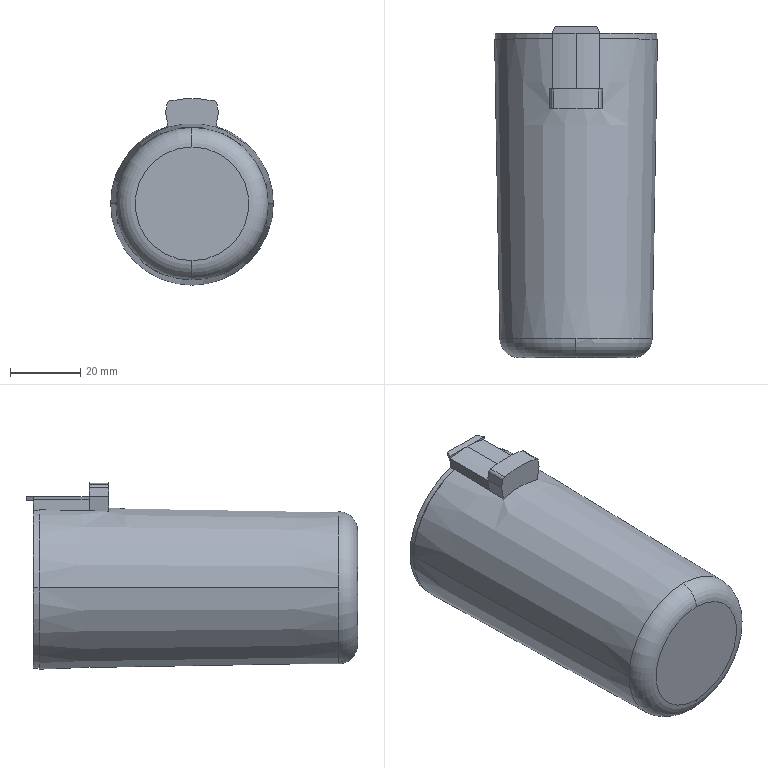Part | SolidWorks | features BaseBody 1 | 1 solid | 30 faces | box 46.4 x 94.4 x 53.2 mm | volume 146390 mm3 | plane 18 | cylinder 8 | torus 2 | cone 2 | commonest cylinder face diameters 46 x3 2 x2 51.98 x2 60 x1
STEP:
#1=CARTESIAN_POINT('',(21.709,-118.996,0.));
#2=VERTEX_POINT('',#1);
#3=CARTESIAN_POINT('',(0.,-118.996,21.709));
#4=VERTEX_POINT('',#3);
#5=CARTESIAN_POINT('',(0.,-118.996,0.));
#6=DIRECTION('',(0.,-1.,0.));
#7=DIRECTION('',(0.,0.,-1.));
#8=AXIS2_PLACEMENT_3D('',#5,#6,#7);
#9=CIRCLE('',#8,21.709);
#10=EDGE_CURVE('',#2,#4,#9,.T.);
#11=ORIENTED_EDGE('',*,*,#10,.T.);
#12=CARTESIAN_POINT('',(0.,-124.4,16.21));
#13=VERTEX_POINT('',#12);
#14=CARTESIAN_POINT('',(0.,-118.9,16.21));
#15=DIRECTION('',(1.,0.,0.));
#16=DIRECTION('',(0.,0.,-1.));
#17=AXIS2_PLACEMENT_3D('',#14,#15,#16);
#18=CIRCLE('',#17,5.5);
#19=EDGE_CURVE('',#4,#13,#18,.T.);
#20=ORIENTED_EDGE('',*,*,#19,.T.);
#21=CARTESIAN_POINT('',(0.,-124.4,-16.21));
#22=VERTEX_POINT('',#21);
#23=CARTESIAN_POINT('',(0.,-124.4,0.));
#24=DIRECTION('',(0.,-1.,0.));
#25=DIRECTION('',(0.,0.,-1.));
#26=AXIS2_PLACEMENT_3D('',#23,#24,#25);
#27=CIRCLE('',#26,16.21);
#28=EDGE_CURVE('',#22,#13,#27,.T.);
#29=ORIENTED_EDGE('',*,*,#28,.F.);
#30=CARTESIAN_POINT('',(0.,-118.996,-21.709));
#31=VERTEX_POINT('',#30);
#32=CARTESIAN_POINT('',(0.,-118.9,-16.21));
#33=DIRECTION('',(-1.,0.,0.));
#34=DIRECTION('',(0.,0.,1.));
#35=AXIS2_PLACEMENT_3D('',#32,#33,#34);
#36=CIRCLE('',#35,5.5);
#37=EDGE_CURVE('',#31,#22,#36,.T.);
#38=ORIENTED_EDGE('',*,*,#37,.F.);
#39=CARTESIAN_POINT('',(0.,-118.996,0.));
#40=DIRECTION('',(0.,-1.,0.));
#41=DIRECTION('',(0.,0.,-1.));
#42=AXIS2_PLACEMENT_3D('',#39,#40,#41);
#43=CIRCLE('',#42,21.709);
#44=EDGE_CURVE('',#31,#2,#43,.T.);
#45=ORIENTED_EDGE('',*,*,#44,.T.);
#46=EDGE_LOOP('',(#11,#20,#29,#38,#45));
#47=FACE_OUTER_BOUND('',#46,.T.);
#48=CARTESIAN_POINT('',(0.,-118.9,0.));
#49=DIRECTION('',(0.,-1.,0.));
#50=DIRECTION('',(0.,0.,-1.));
#51=AXIS2_PLACEMENT_3D('',#48,#49,#50);
#52=TOROIDAL_SURFACE('',#51,16.21,5.5);
#53=ADVANCED_FACE('',(#47),#52,.T.);
#54=ORIENTED_EDGE('',*,*,#10,.F.);
#55=CARTESIAN_POINT('',(23.2,-33.6,0.));
#56=VERTEX_POINT('',#55);
#57=CARTESIAN_POINT('',(23.2,-33.6,0.));
#58=DIRECTION('',(0.01745,0.9998,0.));
#59=VECTOR('',#58,1000.);
#60=LINE('',#57,#59);
#61=EDGE_CURVE('',#2,#56,#60,.T.);
#62=ORIENTED_EDGE('',*,*,#61,.T.);
#63=CARTESIAN_POINT('',(6.7,-33.6,22.211));
#64=VERTEX_POINT('',#63);
#65=CARTESIAN_POINT('',(0.,-33.6,0.));
#66=DIRECTION('',(0.,-1.,0.));
#67=DIRECTION('',(-0.2888,0.,0.9574));
#68=AXIS2_PLACEMENT_3D('',#65,#66,#67);
#69=CIRCLE('',#68,23.2);
#70=EDGE_CURVE('',#56,#64,#69,.T.);
#71=ORIENTED_EDGE('',*,*,#70,.T.);
#72=CARTESIAN_POINT('',(6.7,-47.862,21.951));
#73=VERTEX_POINT('',#72);
#74=CARTESIAN_POINT('',(6.7,-33.6,22.211));
#75=CARTESIAN_POINT('',(6.7,-38.354,22.125));
#76=CARTESIAN_POINT('',(6.7,-43.108,22.038));
#77=CARTESIAN_POINT('',(6.7,-47.862,21.951));
#78=B_SPLINE_CURVE_WITH_KNOTS('',3,(#74,#75,#76,#77),.UNSPECIFIED.,.F.,.F.,(4,4),(20.375,34.639),.UNSPECIFIED.);
#79=EDGE_CURVE('',#64,#73,#78,.T.);
#80=ORIENTED_EDGE('',*,*,#79,.T.);
#81=CARTESIAN_POINT('',(6.8,-47.862,21.92));
#82=VERTEX_POINT('',#81);
#83=CARTESIAN_POINT('',(0.,-47.862,0.));
#84=DIRECTION('',(0.,1.,0.));
#85=DIRECTION('',(0.2919,0.,0.9564));
#86=AXIS2_PLACEMENT_3D('',#83,#84,#85);
#87=CIRCLE('',#86,22.951);
#88=EDGE_CURVE('',#73,#82,#87,.T.);
#89=ORIENTED_EDGE('',*,*,#88,.T.);
#90=CARTESIAN_POINT('',(6.782,-53.5,21.823));
#91=VERTEX_POINT('',#90);
#92=CARTESIAN_POINT('',(6.782,-53.5,21.823));
#93=CARTESIAN_POINT('',(6.788,-51.621,21.855));
#94=CARTESIAN_POINT('',(6.794,-49.741,21.888));
#95=CARTESIAN_POINT('',(6.8,-47.862,21.92));
#96=B_SPLINE_CURVE_WITH_KNOTS('',3,(#92,#93,#94,#95),.UNSPECIFIED.,.F.,.F.,(4,4),(0.0002,5.639),.UNSPECIFIED.);
#97=EDGE_CURVE('',#91,#82,#96,.T.);
#98=ORIENTED_EDGE('',*,*,#97,.F.);
#99=CARTESIAN_POINT('',(-6.782,-53.5,21.823));
#100=VERTEX_POINT('',#99);
#101=CARTESIAN_POINT('',(0.,-53.5,0.));
#102=DIRECTION('',(0.,1.,0.));
#103=DIRECTION('',(-0.2968,0.,0.9549));
#104=AXIS2_PLACEMENT_3D('',#101,#102,#103);
#105=CIRCLE('',#104,22.853);
#106=EDGE_CURVE('',#100,#91,#105,.T.);
#107=ORIENTED_EDGE('',*,*,#106,.F.);
#108=CARTESIAN_POINT('',(-6.8,-47.862,21.92));
#109=VERTEX_POINT('',#108);
#110=CARTESIAN_POINT('',(-6.8,-47.862,21.92));
#111=CARTESIAN_POINT('',(-6.794,-49.741,21.888));
#112=CARTESIAN_POINT('',(-6.788,-51.621,21.855));
#113=CARTESIAN_POINT('',(-6.782,-53.5,21.823));
#114=B_SPLINE_CURVE_WITH_KNOTS('',3,(#110,#111,#112,#113),.UNSPECIFIED.,.F.,.F.,(4,4),(0.0002,5.639),.UNSPECIFIED.);
#115=EDGE_CURVE('',#109,#100,#114,.T.);
#116=ORIENTED_EDGE('',*,*,#115,.F.);
#117=CARTESIAN_POINT('',(-6.7,-47.862,21.951));
#118=VERTEX_POINT('',#117);
#119=CARTESIAN_POINT('',(0.,-47.862,0.));
#120=DIRECTION('',(0.,1.,0.));
#121=DIRECTION('',(-0.2963,0.,0.9551));
#122=AXIS2_PLACEMENT_3D('',#119,#120,#121);
#123=CIRCLE('',#122,22.951);
#124=EDGE_CURVE('',#109,#118,#123,.T.);
#125=ORIENTED_EDGE('',*,*,#124,.T.);
#126=CARTESIAN_POINT('',(-6.7,-33.6,22.211));
#127=VERTEX_POINT('',#126);
#128=CARTESIAN_POINT('',(-6.7,-47.862,21.951));
#129=CARTESIAN_POINT('',(-6.7,-43.108,22.038));
#130=CARTESIAN_POINT('',(-6.7,-38.354,22.125));
#131=CARTESIAN_POINT('',(-6.7,-33.6,22.211));
#132=B_SPLINE_CURVE_WITH_KNOTS('',3,(#128,#129,#130,#131),.UNSPECIFIED.,.F.,.F.,(4,4),(26.014,40.278),.UNSPECIFIED.);
#133=EDGE_CURVE('',#118,#127,#132,.T.);
#134=ORIENTED_EDGE('',*,*,#133,.T.);
#135=CARTESIAN_POINT('',(-23.2,-33.6,0.));
#136=VERTEX_POINT('',#135);
#137=CARTESIAN_POINT('',(0.,-33.6,0.));
#138=DIRECTION('',(0.,-1.,0.));
#139=DIRECTION('',(-0.2888,0.,0.9574));
#140=AXIS2_PLACEMENT_3D('',#137,#138,#139);
#141=CIRCLE('',#140,23.2);
#142=EDGE_CURVE('',#127,#136,#141,.T.);
#143=ORIENTED_EDGE('',*,*,#142,.T.);
#144=CARTESIAN_POINT('',(-21.709,-118.996,0.));
#145=VERTEX_POINT('',#144);
#146=CARTESIAN_POINT('',(-23.2,-33.6,0.));
#147=DIRECTION('',(-0.01745,0.9998,0.));
#148=VECTOR('',#147,1000.);
#149=LINE('',#146,#148);
#150=EDGE_CURVE('',#145,#136,#149,.T.);
#151=ORIENTED_EDGE('',*,*,#150,.F.);
#152=CARTESIAN_POINT('',(0.,-118.996,0.));
#153=DIRECTION('',(0.,-1.,0.));
#154=DIRECTION('',(0.,0.,-1.));
#155=AXIS2_PLACEMENT_3D('',#152,#153,#154);
#156=CIRCLE('',#155,21.709);
#157=EDGE_CURVE('',#4,#145,#156,.T.);
#158=ORIENTED_EDGE('',*,*,#157,.F.);
#159=EDGE_LOOP('',(#54,#62,#71,#80,#89,#98,#107,#116,#125,#134,#143,#151,#158));
#160=FACE_OUTER_BOUND('',#159,.T.);
#161=CARTESIAN_POINT('',(0.,-33.6,0.));
#162=DIRECTION('',(0.,1.,0.));
#163=DIRECTION('',(-1.,0.,0.));
#164=AXIS2_PLACEMENT_3D('',#161,#162,#163);
#165=CONICAL_SURFACE('',#164,23.2,0.01745);
#166=ADVANCED_FACE('',(#160),#165,.T.);
#167=CARTESIAN_POINT('',(0.,-47.862,25.99));
#168=VERTEX_POINT('',#167);
#169=CARTESIAN_POINT('',(-6.7,-47.862,25.112));
#170=VERTEX_POINT('',#169);
#171=CARTESIAN_POINT('',(0.,-47.862,0.));
#172=DIRECTION('',(0.,-1.,0.));
#173=DIRECTION('',(0.2578,0.,0.9662));
#174=AXIS2_PLACEMENT_3D('',#171,#172,#173);
#175=CIRCLE('',#174,25.99);
#176=EDGE_CURVE('',#168,#170,#175,.T.);
#177=ORIENTED_EDGE('',*,*,#176,.F.);
#178=CARTESIAN_POINT('',(0.,-32.,25.99));
#179=VERTEX_POINT('',#178);
#180=CARTESIAN_POINT('',(0.,-53.5,25.99));
#181=DIRECTION('',(0.,1.,0.));
#182=VECTOR('',#181,1000.);
#183=LINE('',#180,#182);
#184=EDGE_CURVE('',#168,#179,#183,.T.);
#185=ORIENTED_EDGE('',*,*,#184,.T.);
#186=CARTESIAN_POINT('',(-6.7,-32.,25.112));
#187=VERTEX_POINT('',#186);
#188=CARTESIAN_POINT('',(0.,-32.,0.));
#189=DIRECTION('',(0.,1.,0.));
#190=DIRECTION('',(-0.2578,0.,0.9662));
#191=AXIS2_PLACEMENT_3D('',#188,#189,#190);
#192=CIRCLE('',#191,25.99);
#193=EDGE_CURVE('',#187,#179,#192,.T.);
#194=ORIENTED_EDGE('',*,*,#193,.F.);
#195=CARTESIAN_POINT('',(-6.7,-47.862,25.112));
#196=DIRECTION('',(0.,1.,0.));
#197=VECTOR('',#196,1000.);
#198=LINE('',#195,#197);
#199=EDGE_CURVE('',#170,#187,#198,.T.);
#200=ORIENTED_EDGE('',*,*,#199,.F.);
#201=EDGE_LOOP('',(#177,#185,#194,#200));
#202=FACE_OUTER_BOUND('',#201,.T.);
#203=CARTESIAN_POINT('',(0.,-53.5,0.));
#204=DIRECTION('',(0.,1.,0.));
#205=DIRECTION('',(0.,0.,1.));
#206=AXIS2_PLACEMENT_3D('',#203,#204,#205);
#207=CYLINDRICAL_SURFACE('',#206,25.99);
#208=ADVANCED_FACE('',(#202),#207,.T.);
#209=CARTESIAN_POINT('',(-6.7,-32.,22.002));
#210=VERTEX_POINT('',#209);
#211=CARTESIAN_POINT('',(-23.,-32.,0.));
#212=VERTEX_POINT('',#211);
#213=CARTESIAN_POINT('',(0.,-32.,0.));
#214=DIRECTION('',(0.,-1.,0.));
#215=DIRECTION('',(-0.2913,0.,0.9566));
#216=AXIS2_PLACEMENT_3D('',#213,#214,#215);
#217=CIRCLE('',#216,23.);
#218=EDGE_CURVE('',#210,#212,#217,.T.);
#219=ORIENTED_EDGE('',*,*,#218,.T.);
#220=CARTESIAN_POINT('',(-23.,-33.6,0.));
#221=VERTEX_POINT('',#220);
#222=CARTESIAN_POINT('',(-23.,-104.3,0.));
#223=DIRECTION('',(0.,-1.,0.));
#224=VECTOR('',#223,1000.);
#225=LINE('',#222,#224);
#226=EDGE_CURVE('',#212,#221,#225,.T.);
#227=ORIENTED_EDGE('',*,*,#226,.T.);
#228=CARTESIAN_POINT('',(-6.7,-33.6,22.002));
#229=VERTEX_POINT('',#228);
#230=CARTESIAN_POINT('',(0.,-33.6,0.));
#231=DIRECTION('',(0.,-1.,0.));
#232=DIRECTION('',(-0.2913,0.,0.9566));
#233=AXIS2_PLACEMENT_3D('',#230,#231,#232);
#234=CIRCLE('',#233,23.);
#235=EDGE_CURVE('',#229,#221,#234,.T.);
#236=ORIENTED_EDGE('',*,*,#235,.F.);
#237=CARTESIAN_POINT('',(-6.7,-33.6,22.002));
#238=DIRECTION('',(0.,1.,0.));
#239=VECTOR('',#238,1000.);
#240=LINE('',#237,#239);
#241=EDGE_CURVE('',#229,#210,#240,.T.);
#242=ORIENTED_EDGE('',*,*,#241,.T.);
#243=EDGE_LOOP('',(#219,#227,#236,#242));
#244=FACE_OUTER_BOUND('',#243,.T.);
#245=CARTESIAN_POINT('',(0.,-104.3,0.));
#246=DIRECTION('',(0.,-1.,0.));
#247=DIRECTION('',(1.,0.,0.));
#248=AXIS2_PLACEMENT_3D('',#245,#246,#247);
#249=CYLINDRICAL_SURFACE('',#248,23.);
#250=ADVANCED_FACE('',(#244),#249,.T.);
#251=ORIENTED_EDGE('',*,*,#226,.F.);
#252=CARTESIAN_POINT('',(23.,-32.,0.));
#253=VERTEX_POINT('',#252);
#254=CARTESIAN_POINT('',(0.,-32.,0.));
#255=DIRECTION('',(0.,-1.,0.));
#256=DIRECTION('',(-0.2913,0.,0.9566));
#257=AXIS2_PLACEMENT_3D('',#254,#255,#256);
#258=CIRCLE('',#257,23.);
#259=EDGE_CURVE('',#212,#253,#258,.T.);
#260=ORIENTED_EDGE('',*,*,#259,.T.);
#261=CARTESIAN_POINT('',(23.,-33.6,0.));
#262=VERTEX_POINT('',#261);
#263=CARTESIAN_POINT('',(23.,-104.3,0.));
#264=DIRECTION('',(0.,-1.,0.));
#265=VECTOR('',#264,1000.);
#266=LINE('',#263,#265);
#267=EDGE_CURVE('',#253,#262,#266,.T.);
#268=ORIENTED_EDGE('',*,*,#267,.T.);
#269=CARTESIAN_POINT('',(0.,-33.6,0.));
#270=DIRECTION('',(0.,-1.,0.));
#271=DIRECTION('',(-0.2913,0.,0.9566));
#272=AXIS2_PLACEMENT_3D('',#269,#270,#271);
#273=CIRCLE('',#272,23.);
#274=EDGE_CURVE('',#221,#262,#273,.T.);
#275=ORIENTED_EDGE('',*,*,#274,.F.);
#276=EDGE_LOOP('',(#251,#260,#268,#275));
#277=FACE_OUTER_BOUND('',#276,.T.);
#278=CARTESIAN_POINT('',(0.,-104.3,0.));
#279=DIRECTION('',(0.,-1.,0.));
#280=DIRECTION('',(1.,0.,0.));
#281=AXIS2_PLACEMENT_3D('',#278,#279,#280);
#282=CYLINDRICAL_SURFACE('',#281,23.);
#283=ADVANCED_FACE('',(#277),#282,.T.);
#284=ORIENTED_EDGE('',*,*,#218,.F.);
#285=CARTESIAN_POINT('',(-6.7,-32.,24.79));
#286=VERTEX_POINT('',#285);
#287=CARTESIAN_POINT('',(-6.7,-32.,22.002));
#288=DIRECTION('',(0.,0.,1.));
#289=VECTOR('',#288,1000.);
#290=LINE('',#287,#289);
#291=EDGE_CURVE('',#210,#286,#290,.T.);
#292=ORIENTED_EDGE('',*,*,#291,.T.);
#293=CARTESIAN_POINT('',(6.7,-32.,24.79));
#294=VERTEX_POINT('',#293);
#295=CARTESIAN_POINT('',(-6.7,-32.,24.79));
#296=DIRECTION('',(1.,0.,0.));
#297=VECTOR('',#296,1000.);
#298=LINE('',#295,#297);
#299=EDGE_CURVE('',#286,#294,#298,.T.);
#300=ORIENTED_EDGE('',*,*,#299,.T.);
#301=CARTESIAN_POINT('',(6.7,-32.,22.002));
#302=VERTEX_POINT('',#301);
#303=CARTESIAN_POINT('',(6.7,-32.,24.79));
#304=DIRECTION('',(0.,0.,-1.));
#305=VECTOR('',#304,1000.);
#306=LINE('',#303,#305);
#307=EDGE_CURVE('',#294,#302,#306,.T.);
#308=ORIENTED_EDGE('',*,*,#307,.T.);
#309=CARTESIAN_POINT('',(0.,-32.,0.));
#310=DIRECTION('',(0.,-1.,0.));
#311=DIRECTION('',(-0.2913,0.,0.9566));
#312=AXIS2_PLACEMENT_3D('',#309,#310,#311);
#313=CIRCLE('',#312,23.);
#314=EDGE_CURVE('',#253,#302,#313,.T.);
#315=ORIENTED_EDGE('',*,*,#314,.F.);
#316=ORIENTED_EDGE('',*,*,#259,.F.);
#317=EDGE_LOOP('',(#284,#292,#300,#308,#315,#316));
#318=FACE_OUTER_BOUND('',#317,.T.);
#319=CARTESIAN_POINT('',(0.,-32.,0.));
#320=DIRECTION('',(0.,-1.,0.));
#321=DIRECTION('',(1.,0.,0.));
#322=AXIS2_PLACEMENT_3D('',#319,#320,#321);
#323=PLANE('',#322);
#324=ADVANCED_FACE('',(#318),#323,.F.);
#325=ORIENTED_EDGE('',*,*,#267,.F.);
#326=ORIENTED_EDGE('',*,*,#314,.T.);
#327=CARTESIAN_POINT('',(6.7,-33.6,22.002));
#328=VERTEX_POINT('',#327);
#329=CARTESIAN_POINT('',(6.7,-32.,22.002));
#330=DIRECTION('',(0.,-1.,0.));
#331=VECTOR('',#330,1000.);
#332=LINE('',#329,#331);
#333=EDGE_CURVE('',#302,#328,#332,.T.);
#334=ORIENTED_EDGE('',*,*,#333,.T.);
#335=CARTESIAN_POINT('',(0.,-33.6,0.));
#336=DIRECTION('',(0.,-1.,0.));
#337=DIRECTION('',(-0.2913,0.,0.9566));
#338=AXIS2_PLACEMENT_3D('',#335,#336,#337);
#339=CIRCLE('',#338,23.);
#340=EDGE_CURVE('',#262,#328,#339,.T.);
#341=ORIENTED_EDGE('',*,*,#340,.F.);
#342=EDGE_LOOP('',(#325,#326,#334,#341));
#343=FACE_OUTER_BOUND('',#342,.T.);
#344=CARTESIAN_POINT('',(0.,-104.3,0.));
#345=DIRECTION('',(0.,-1.,0.));
#346=DIRECTION('',(1.,0.,0.));
#347=AXIS2_PLACEMENT_3D('',#344,#345,#346);
#348=CYLINDRICAL_SURFACE('',#347,23.);
#349=ADVANCED_FACE('',(#343),#348,.T.);
#350=CARTESIAN_POINT('',(-6.7,-47.862,25.112));
#351=DIRECTION('',(0.,0.,-1.));
#352=VECTOR('',#351,1000.);
#353=LINE('',#350,#352);
#354=EDGE_CURVE('',#170,#118,#353,.T.);
#355=ORIENTED_EDGE('',*,*,#354,.F.);
#356=ORIENTED_EDGE('',*,*,#199,.T.);
#357=CARTESIAN_POINT('',(-6.7,-32.,24.79));
#358=DIRECTION('',(0.,0.,1.));
#359=VECTOR('',#358,1000.);
#360=LINE('',#357,#359);
#361=EDGE_CURVE('',#286,#187,#360,.T.);
#362=ORIENTED_EDGE('',*,*,#361,.F.);
#363=ORIENTED_EDGE('',*,*,#291,.F.);
#364=ORIENTED_EDGE('',*,*,#241,.F.);
#365=CARTESIAN_POINT('',(-6.7,-33.6,22.211));
#366=DIRECTION('',(0.,0.,-1.));
#367=VECTOR('',#366,1000.);
#368=LINE('',#365,#367);
#369=EDGE_CURVE('',#127,#229,#368,.T.);
#370=ORIENTED_EDGE('',*,*,#369,.F.);
#371=ORIENTED_EDGE('',*,*,#133,.F.);
#372=EDGE_LOOP('',(#355,#356,#362,#363,#364,#370,#371));
#373=FACE_OUTER_BOUND('',#372,.T.);
#374=CARTESIAN_POINT('',(-6.7,-53.5,18.844));
#375=DIRECTION('',(-1.,0.,0.));
#376=DIRECTION('',(0.,0.,1.));
#377=AXIS2_PLACEMENT_3D('',#374,#375,#376);
#378=PLANE('',#377);
#379=ADVANCED_FACE('',(#373),#378,.T.);
#380=CARTESIAN_POINT('',(-5.845,-30.,24.79));
#381=VERTEX_POINT('',#380);
#382=CARTESIAN_POINT('',(-7.,-32.,24.79));
#383=VERTEX_POINT('',#382);
#384=CARTESIAN_POINT('',(-5.845,-30.,24.79));
#385=DIRECTION('',(-0.5,-0.866,0.));
#386=VECTOR('',#385,1000.);
#387=LINE('',#384,#386);
#388=EDGE_CURVE('',#381,#383,#387,.T.);
#389=ORIENTED_EDGE('',*,*,#388,.F.);
#390=CARTESIAN_POINT('',(5.845,-30.,24.79));
#391=VERTEX_POINT('',#390);
#392=CARTESIAN_POINT('',(5.845,-30.,24.79));
#393=DIRECTION('',(-1.,0.,0.));
#394=VECTOR('',#393,1000.);
#395=LINE('',#392,#394);
#396=EDGE_CURVE('',#391,#381,#395,.T.);
#397=ORIENTED_EDGE('',*,*,#396,.F.);
#398=CARTESIAN_POINT('',(7.,-32.,24.79));
#399=VERTEX_POINT('',#398);
#400=CARTESIAN_POINT('',(7.,-32.,24.79));
#401=DIRECTION('',(-0.5,0.866,0.));
#402=VECTOR('',#401,1000.);
#403=LINE('',#400,#402);
#404=EDGE_CURVE('',#399,#391,#403,.T.);
#405=ORIENTED_EDGE('',*,*,#404,.F.);
#406=CARTESIAN_POINT('',(6.7,-32.,24.79));
#407=DIRECTION('',(1.,0.,0.));
#408=VECTOR('',#407,1000.);
#409=LINE('',#406,#408);
#410=EDGE_CURVE('',#294,#399,#409,.T.);
#411=ORIENTED_EDGE('',*,*,#410,.F.);
#412=ORIENTED_EDGE('',*,*,#299,.F.);
#413=CARTESIAN_POINT('',(-7.,-32.,24.79));
#414=DIRECTION('',(1.,0.,0.));
#415=VECTOR('',#414,1000.);
#416=LINE('',#413,#415);
#417=EDGE_CURVE('',#383,#286,#416,.T.);
#418=ORIENTED_EDGE('',*,*,#417,.F.);
#419=EDGE_LOOP('',(#389,#397,#405,#411,#412,#418));
#420=FACE_OUTER_BOUND('',#419,.T.);
#421=CARTESIAN_POINT('',(0.,0.,24.79));
#422=DIRECTION('',(0.,0.,1.));
#423=DIRECTION('',(1.,0.,0.));
#424=AXIS2_PLACEMENT_3D('',#421,#422,#423);
#425=PLANE('',#424);
#426=ADVANCED_FACE('',(#420),#425,.F.);
#427=CARTESIAN_POINT('',(6.7,-47.862,25.112));
#428=VERTEX_POINT('',#427);
#429=CARTESIAN_POINT('',(6.7,-47.862,21.951));
#430=DIRECTION('',(0.,0.,1.));
#431=VECTOR('',#430,1000.);
#432=LINE('',#429,#431);
#433=EDGE_CURVE('',#73,#428,#432,.T.);
#434=ORIENTED_EDGE('',*,*,#433,.F.);
#435=ORIENTED_EDGE('',*,*,#79,.F.);
#436=CARTESIAN_POINT('',(6.7,-33.6,22.002));
#437=DIRECTION('',(0.,0.,1.));
#438=VECTOR('',#437,1000.);
#439=LINE('',#436,#438);
#440=EDGE_CURVE('',#328,#64,#439,.T.);
#441=ORIENTED_EDGE('',*,*,#440,.F.);
#442=ORIENTED_EDGE('',*,*,#333,.F.);
#443=ORIENTED_EDGE('',*,*,#307,.F.);
#444=CARTESIAN_POINT('',(6.7,-32.,25.112));
#445=VERTEX_POINT('',#444);
#446=CARTESIAN_POINT('',(6.7,-32.,25.112));
#447=DIRECTION('',(0.,0.,-1.));
#448=VECTOR('',#447,1000.);
#449=LINE('',#446,#448);
#450=EDGE_CURVE('',#445,#294,#449,.T.);
#451=ORIENTED_EDGE('',*,*,#450,.F.);
#452=CARTESIAN_POINT('',(6.7,-47.862,25.112));
#453=DIRECTION('',(0.,1.,0.));
#454=VECTOR('',#453,1000.);
#455=LINE('',#452,#454);
#456=EDGE_CURVE('',#428,#445,#455,.T.);
#457=ORIENTED_EDGE('',*,*,#456,.F.);
#458=EDGE_LOOP('',(#434,#435,#441,#442,#443,#451,#457));
#459=FACE_OUTER_BOUND('',#458,.T.);
#460=CARTESIAN_POINT('',(6.7,-53.5,25.112));
#461=DIRECTION('',(1.,0.,0.));
#462=DIRECTION('',(0.,0.,-1.));
#463=AXIS2_PLACEMENT_3D('',#460,#461,#462);
#464=PLANE('',#463);
#465=ADVANCED_FACE('',(#459),#464,.T.);
#466=ORIENTED_EDGE('',*,*,#142,.F.);
#467=ORIENTED_EDGE('',*,*,#369,.T.);
#468=ORIENTED_EDGE('',*,*,#235,.T.);
#469=ORIENTED_EDGE('',*,*,#274,.T.);
#470=ORIENTED_EDGE('',*,*,#340,.T.);
#471=ORIENTED_EDGE('',*,*,#440,.T.);
#472=ORIENTED_EDGE('',*,*,#70,.F.);
#473=CARTESIAN_POINT('',(0.,-33.6,0.));
#474=DIRECTION('',(0.,-1.,0.));
#475=DIRECTION('',(-0.2888,0.,0.9574));
#476=AXIS2_PLACEMENT_3D('',#473,#474,#475);
#477=CIRCLE('',#476,23.2);
#478=EDGE_CURVE('',#136,#56,#477,.T.);
#479=ORIENTED_EDGE('',*,*,#478,.F.);
#480=EDGE_LOOP('',(#466,#467,#468,#469,#470,#471,#472,#479));
#481=FACE_OUTER_BOUND('',#480,.T.);
#482=CARTESIAN_POINT('',(23.,-33.6,0.));
#483=DIRECTION('',(0.,-1.,0.));
#484=DIRECTION('',(1.,0.,0.));
#485=AXIS2_PLACEMENT_3D('',#482,#483,#484);
#486=PLANE('',#485);
#487=ADVANCED_FACE('',(#481),#486,.F.);
#488=ORIENTED_EDGE('',*,*,#88,.F.);
#489=ORIENTED_EDGE('',*,*,#433,.T.);
#490=CARTESIAN_POINT('',(0.,-47.862,0.));
#491=DIRECTION('',(0.,-1.,0.));
#492=DIRECTION('',(0.2578,0.,0.9662));
#493=AXIS2_PLACEMENT_3D('',#490,#491,#492);
#494=CIRCLE('',#493,25.99);
#495=EDGE_CURVE('',#428,#168,#494,.T.);
#496=ORIENTED_EDGE('',*,*,#495,.T.);
#497=ORIENTED_EDGE('',*,*,#176,.T.);
#498=ORIENTED_EDGE('',*,*,#354,.T.);
#499=ORIENTED_EDGE('',*,*,#124,.F.);
#500=CARTESIAN_POINT('',(-7.555,-47.862,26.024));
#501=VERTEX_POINT('',#500);
#502=CARTESIAN_POINT('',(-6.8,-47.862,21.92));
#503=DIRECTION('',(-0.1808,0.,0.9835));
#504=VECTOR('',#503,1000.);
#505=LINE('',#502,#504);
#506=EDGE_CURVE('',#109,#501,#505,.T.);
#507=ORIENTED_EDGE('',*,*,#506,.T.);
#508=CARTESIAN_POINT('',(-7.115,-47.862,28.518));
#509=VERTEX_POINT('',#508);
#510=CARTESIAN_POINT('',(-7.555,-47.862,26.024));
#511=DIRECTION('',(0.1736,0.,0.9848));
#512=VECTOR('',#511,1000.);
#513=LINE('',#510,#512);
#514=EDGE_CURVE('',#501,#509,#513,.T.);
#515=ORIENTED_EDGE('',*,*,#514,.T.);
#516=CARTESIAN_POINT('',(-6.342,-47.862,29.322));
#517=VERTEX_POINT('',#516);
#518=CARTESIAN_POINT('',(-6.13,-47.862,28.345));
#519=DIRECTION('',(0.,1.,0.));
#520=DIRECTION('',(-0.9848,0.,0.1736));
#521=AXIS2_PLACEMENT_3D('',#518,#519,#520);
#522=CIRCLE('',#521,1.);
#523=EDGE_CURVE('',#509,#517,#522,.T.);
#524=ORIENTED_EDGE('',*,*,#523,.T.);
#525=CARTESIAN_POINT('',(6.342,-47.862,29.322));
#526=VERTEX_POINT('',#525);
#527=CARTESIAN_POINT('',(0.,-47.862,0.));
#528=DIRECTION('',(0.,1.,0.));
#529=DIRECTION('',(-0.2114,0.,0.9774));
#530=AXIS2_PLACEMENT_3D('',#527,#528,#529);
#531=CIRCLE('',#530,30.);
#532=EDGE_CURVE('',#517,#526,#531,.T.);
#533=ORIENTED_EDGE('',*,*,#532,.T.);
#534=CARTESIAN_POINT('',(7.115,-47.862,28.518));
#535=VERTEX_POINT('',#534);
#536=CARTESIAN_POINT('',(6.13,-47.862,28.345));
#537=DIRECTION('',(0.,1.,0.));
#538=DIRECTION('',(0.2114,0.,0.9774));
#539=AXIS2_PLACEMENT_3D('',#536,#537,#538);
#540=CIRCLE('',#539,1.);
#541=EDGE_CURVE('',#526,#535,#540,.T.);
#542=ORIENTED_EDGE('',*,*,#541,.T.);
#543=CARTESIAN_POINT('',(7.555,-47.862,26.024));
#544=VERTEX_POINT('',#543);
#545=CARTESIAN_POINT('',(7.115,-47.862,28.518));
#546=DIRECTION('',(0.1736,0.,-0.9848));
#547=VECTOR('',#546,1000.);
#548=LINE('',#545,#547);
#549=EDGE_CURVE('',#535,#544,#548,.T.);
#550=ORIENTED_EDGE('',*,*,#549,.T.);
#551=CARTESIAN_POINT('',(7.555,-47.862,26.024));
#552=DIRECTION('',(-0.1808,0.,-0.9835));
#553=VECTOR('',#552,1000.);
#554=LINE('',#551,#553);
#555=EDGE_CURVE('',#544,#82,#554,.T.);
#556=ORIENTED_EDGE('',*,*,#555,.T.);
#557=EDGE_LOOP('',(#488,#489,#496,#497,#498,#499,#507,#515,#524,#533,#542,#550,#556));
#558=FACE_OUTER_BOUND('',#557,.T.);
#559=CARTESIAN_POINT('',(-6.13,-47.862,28.345));
#560=DIRECTION('',(0.,1.,0.));
#561=DIRECTION('',(0.,0.,1.));
#562=AXIS2_PLACEMENT_3D('',#559,#560,#561);
#563=PLANE('',#562);
#564=ADVANCED_FACE('',(#558),#563,.T.);
#565=ORIENTED_EDGE('',*,*,#184,.F.);
#566=ORIENTED_EDGE('',*,*,#495,.F.);
#567=ORIENTED_EDGE('',*,*,#456,.T.);
#568=CARTESIAN_POINT('',(0.,-32.,0.));
#569=DIRECTION('',(0.,1.,0.));
#570=DIRECTION('',(0.,0.,1.));
#571=AXIS2_PLACEMENT_3D('',#568,#569,#570);
#572=CIRCLE('',#571,25.99);
#573=EDGE_CURVE('',#179,#445,#572,.T.);
#574=ORIENTED_EDGE('',*,*,#573,.F.);
#575=EDGE_LOOP('',(#565,#566,#567,#574));
#576=FACE_OUTER_BOUND('',#575,.T.);
#577=CARTESIAN_POINT('',(0.,-53.5,0.));
#578=DIRECTION('',(0.,1.,0.));
#579=DIRECTION('',(0.,0.,1.));
#580=AXIS2_PLACEMENT_3D('',#577,#578,#579);
#581=CYLINDRICAL_SURFACE('',#580,25.99);
#582=ADVANCED_FACE('',(#576),#581,.T.);
#583=ORIENTED_EDGE('',*,*,#417,.T.);
#584=ORIENTED_EDGE('',*,*,#361,.T.);
#585=ORIENTED_EDGE('',*,*,#193,.T.);
#586=CARTESIAN_POINT('',(-7.,-32.,25.99));
#587=VERTEX_POINT('',#586);
#588=CARTESIAN_POINT('',(-7.,-32.,25.99));
#589=DIRECTION('',(1.,0.,0.));
#590=VECTOR('',#589,1000.);
#591=LINE('',#588,#590);
#592=EDGE_CURVE('',#587,#179,#591,.T.);
#593=ORIENTED_EDGE('',*,*,#592,.F.);
#594=CARTESIAN_POINT('',(-7.,-32.,24.79));
#595=DIRECTION('',(0.,0.,1.));
#596=VECTOR('',#595,1000.);
#597=LINE('',#594,#596);
#598=EDGE_CURVE('',#383,#587,#597,.T.);
#599=ORIENTED_EDGE('',*,*,#598,.F.);
#600=EDGE_LOOP('',(#583,#584,#585,#593,#599));
#601=FACE_OUTER_BOUND('',#600,.T.);
#602=CARTESIAN_POINT('',(-7.,-32.,24.79));
#603=DIRECTION('',(0.,-1.,0.));
#604=DIRECTION('',(0.,0.,-1.));
#605=AXIS2_PLACEMENT_3D('',#602,#603,#604);
#606=PLANE('',#605);
#607=ADVANCED_FACE('',(#601),#606,.T.);
#608=ORIENTED_EDGE('',*,*,#61,.F.);
#609=ORIENTED_EDGE('',*,*,#44,.F.);
#610=CARTESIAN_POINT('',(0.,-118.996,0.));
#611=DIRECTION('',(0.,-1.,0.));
#612=DIRECTION('',(0.,0.,-1.));
#613=AXIS2_PLACEMENT_3D('',#610,#611,#612);
#614=CIRCLE('',#613,21.709);
#615=EDGE_CURVE('',#145,#31,#614,.T.);
#616=ORIENTED_EDGE('',*,*,#615,.F.);
#617=ORIENTED_EDGE('',*,*,#150,.T.);
#618=ORIENTED_EDGE('',*,*,#478,.T.);
#619=EDGE_LOOP('',(#608,#609,#616,#617,#618));
#620=FACE_OUTER_BOUND('',#619,.T.);
#621=CARTESIAN_POINT('',(0.,-33.6,0.));
#622=DIRECTION('',(0.,1.,0.));
#623=DIRECTION('',(-1.,0.,0.));
#624=AXIS2_PLACEMENT_3D('',#621,#622,#623);
#625=CONICAL_SURFACE('',#624,23.2,0.01745);
#626=ADVANCED_FACE('',(#620),#625,.T.);
#627=CARTESIAN_POINT('',(-5.845,-30.,25.99));
#628=VERTEX_POINT('',#627);
#629=CARTESIAN_POINT('',(-5.845,-30.,25.99));
#630=DIRECTION('',(-0.5,-0.866,0.));
#631=VECTOR('',#630,1000.);
#632=LINE('',#629,#631);
#633=EDGE_CURVE('',#628,#587,#632,.T.);
#634=ORIENTED_EDGE('',*,*,#633,.F.);
#635=CARTESIAN_POINT('',(-5.845,-30.,24.79));
#636=DIRECTION('',(0.,0.,1.));
#637=VECTOR('',#636,1000.);
#638=LINE('',#635,#637);
#639=EDGE_CURVE('',#381,#628,#638,.T.);
#640=ORIENTED_EDGE('',*,*,#639,.F.);
#641=ORIENTED_EDGE('',*,*,#388,.T.);
#642=ORIENTED_EDGE('',*,*,#598,.T.);
#643=EDGE_LOOP('',(#634,#640,#641,#642));
#644=FACE_OUTER_BOUND('',#643,.T.);
#645=CARTESIAN_POINT('',(-5.845,-30.,24.79));
#646=DIRECTION('',(-0.866,0.5,0.));
#647=DIRECTION('',(-0.5,-0.866,0.));
#648=AXIS2_PLACEMENT_3D('',#645,#646,#647);
#649=PLANE('',#648);
#650=ADVANCED_FACE('',(#644),#649,.T.);
#651=CARTESIAN_POINT('',(5.845,-30.,25.99));
#652=VERTEX_POINT('',#651);
#653=CARTESIAN_POINT('',(5.845,-30.,25.99));
#654=DIRECTION('',(-1.,0.,0.));
#655=VECTOR('',#654,1000.);
#656=LINE('',#653,#655);
#657=EDGE_CURVE('',#652,#628,#656,.T.);
#658=ORIENTED_EDGE('',*,*,#657,.F.);
#659=CARTESIAN_POINT('',(5.845,-30.,24.79));
#660=DIRECTION('',(0.,0.,1.));
#661=VECTOR('',#660,1000.);
#662=LINE('',#659,#661);
#663=EDGE_CURVE('',#391,#652,#662,.T.);
#664=ORIENTED_EDGE('',*,*,#663,.F.);
#665=ORIENTED_EDGE('',*,*,#396,.T.);
#666=ORIENTED_EDGE('',*,*,#639,.T.);
#667=EDGE_LOOP('',(#658,#664,#665,#666));
#668=FACE_OUTER_BOUND('',#667,.T.);
#669=CARTESIAN_POINT('',(5.845,-30.,24.79));
#670=DIRECTION('',(0.,1.,0.));
#671=DIRECTION('',(0.,0.,1.));
#672=AXIS2_PLACEMENT_3D('',#669,#670,#671);
#673=PLANE('',#672);
#674=ADVANCED_FACE('',(#668),#673,.T.);
#675=CARTESIAN_POINT('',(7.,-32.,25.99));
#676=VERTEX_POINT('',#675);
#677=CARTESIAN_POINT('',(7.,-32.,25.99));
#678=DIRECTION('',(-0.5,0.866,0.));
#679=VECTOR('',#678,1000.);
#680=LINE('',#677,#679);
#681=EDGE_CURVE('',#676,#652,#680,.T.);
#682=ORIENTED_EDGE('',*,*,#681,.F.);
#683=CARTESIAN_POINT('',(7.,-32.,24.79));
#684=DIRECTION('',(0.,0.,1.));
#685=VECTOR('',#684,1000.);
#686=LINE('',#683,#685);
#687=EDGE_CURVE('',#399,#676,#686,.T.);
#688=ORIENTED_EDGE('',*,*,#687,.F.);
#689=ORIENTED_EDGE('',*,*,#404,.T.);
#690=ORIENTED_EDGE('',*,*,#663,.T.);
#691=EDGE_LOOP('',(#682,#688,#689,#690));
#692=FACE_OUTER_BOUND('',#691,.T.);
#693=CARTESIAN_POINT('',(7.,-32.,24.79));
#694=DIRECTION('',(0.866,0.5,0.));
#695=DIRECTION('',(-0.5,0.866,0.));
#696=AXIS2_PLACEMENT_3D('',#693,#694,#695);
#697=PLANE('',#696);
#698=ADVANCED_FACE('',(#692),#697,.T.);
#699=ORIENTED_EDGE('',*,*,#573,.T.);
#700=ORIENTED_EDGE('',*,*,#450,.T.);
#701=ORIENTED_EDGE('',*,*,#410,.T.);
#702=ORIENTED_EDGE('',*,*,#687,.T.);
#703=CARTESIAN_POINT('',(0.,-32.,25.99));
#704=DIRECTION('',(1.,0.,0.));
#705=VECTOR('',#704,1000.);
#706=LINE('',#703,#705);
#707=EDGE_CURVE('',#179,#676,#706,.T.);
#708=ORIENTED_EDGE('',*,*,#707,.F.);
#709=EDGE_LOOP('',(#699,#700,#701,#702,#708));
#710=FACE_OUTER_BOUND('',#709,.T.);
#711=CARTESIAN_POINT('',(-7.,-32.,24.79));
#712=DIRECTION('',(0.,-1.,0.));
#713=DIRECTION('',(0.,0.,-1.));
#714=AXIS2_PLACEMENT_3D('',#711,#712,#713);
#715=PLANE('',#714);
#716=ADVANCED_FACE('',(#710),#715,.T.);
#717=ORIENTED_EDGE('',*,*,#506,.F.);
#718=ORIENTED_EDGE('',*,*,#115,.T.);
#719=CARTESIAN_POINT('',(-7.555,-53.5,26.024));
#720=VERTEX_POINT('',#719);
#721=CARTESIAN_POINT('',(-6.782,-53.5,21.823));
#722=DIRECTION('',(-0.1808,0.,0.9835));
#723=VECTOR('',#722,1000.);
#724=LINE('',#721,#723);
#725=EDGE_CURVE('',#100,#720,#724,.T.);
#726=ORIENTED_EDGE('',*,*,#725,.T.);
#727=CARTESIAN_POINT('',(-7.555,-47.862,26.024));
#728=DIRECTION('',(0.,-1.,0.));
#729=VECTOR('',#728,1000.);
#730=LINE('',#727,#729);
#731=EDGE_CURVE('',#501,#720,#730,.T.);
#732=ORIENTED_EDGE('',*,*,#731,.F.);
#733=EDGE_LOOP('',(#717,#718,#726,#732));
#734=FACE_OUTER_BOUND('',#733,.T.);
#735=CARTESIAN_POINT('',(-6.7,-47.862,21.375));
#736=DIRECTION('',(0.9835,0.,0.1808));
#737=DIRECTION('',(0.1808,0.,-0.9835));
#738=AXIS2_PLACEMENT_3D('',#735,#736,#737);
#739=PLANE('',#738);
#740=ADVANCED_FACE('',(#734),#739,.F.);
#741=CARTESIAN_POINT('',(-7.115,-53.5,28.518));
#742=VERTEX_POINT('',#741);
#743=CARTESIAN_POINT('',(-7.555,-53.5,26.024));
#744=DIRECTION('',(0.1736,0.,0.9848));
#745=VECTOR('',#744,1000.);
#746=LINE('',#743,#745);
#747=EDGE_CURVE('',#720,#742,#746,.T.);
#748=ORIENTED_EDGE('',*,*,#747,.T.);
#749=CARTESIAN_POINT('',(-7.115,-47.862,28.518));
#750=DIRECTION('',(0.,-1.,0.));
#751=VECTOR('',#750,1000.);
#752=LINE('',#749,#751);
#753=EDGE_CURVE('',#509,#742,#752,.T.);
#754=ORIENTED_EDGE('',*,*,#753,.F.);
#755=ORIENTED_EDGE('',*,*,#514,.F.);
#756=ORIENTED_EDGE('',*,*,#731,.T.);
#757=EDGE_LOOP('',(#748,#754,#755,#756));
#758=FACE_OUTER_BOUND('',#757,.T.);
#759=CARTESIAN_POINT('',(-7.555,-47.862,26.024));
#760=DIRECTION('',(0.9848,0.,-0.1736));
#761=DIRECTION('',(-0.1736,0.,-0.9848));
#762=AXIS2_PLACEMENT_3D('',#759,#760,#761);
#763=PLANE('',#762);
#764=ADVANCED_FACE('',(#758),#763,.F.);
#765=CARTESIAN_POINT('',(-6.342,-53.5,29.322));
#766=VERTEX_POINT('',#765);
#767=CARTESIAN_POINT('',(-6.13,-53.5,28.345));
#768=DIRECTION('',(0.,1.,0.));
#769=DIRECTION('',(-0.9848,0.,0.1736));
#770=AXIS2_PLACEMENT_3D('',#767,#768,#769);
#771=CIRCLE('',#770,1.);
#772=EDGE_CURVE('',#742,#766,#771,.T.);
#773=ORIENTED_EDGE('',*,*,#772,.T.);
#774=CARTESIAN_POINT('',(-6.342,-47.862,29.322));
#775=DIRECTION('',(0.,-1.,0.));
#776=VECTOR('',#775,1000.);
#777=LINE('',#774,#776);
#778=EDGE_CURVE('',#517,#766,#777,.T.);
#779=ORIENTED_EDGE('',*,*,#778,.F.);
#780=ORIENTED_EDGE('',*,*,#523,.F.);
#781=ORIENTED_EDGE('',*,*,#753,.T.);
#782=EDGE_LOOP('',(#773,#779,#780,#781));
#783=FACE_OUTER_BOUND('',#782,.T.);
#784=CARTESIAN_POINT('',(-6.13,-47.862,28.345));
#785=DIRECTION('',(0.,-1.,0.));
#786=DIRECTION('',(0.,0.,-1.));
#787=AXIS2_PLACEMENT_3D('',#784,#785,#786);
#788=CYLINDRICAL_SURFACE('',#787,1.);
#789=ADVANCED_FACE('',(#783),#788,.T.);
#790=CARTESIAN_POINT('',(6.342,-53.5,29.322));
#791=VERTEX_POINT('',#790);
#792=CARTESIAN_POINT('',(0.,-53.5,0.));
#793=DIRECTION('',(0.,1.,0.));
#794=DIRECTION('',(-0.2114,0.,0.9774));
#795=AXIS2_PLACEMENT_3D('',#792,#793,#794);
#796=CIRCLE('',#795,30.);
#797=EDGE_CURVE('',#766,#791,#796,.T.);
#798=ORIENTED_EDGE('',*,*,#797,.T.);
#799=CARTESIAN_POINT('',(6.342,-47.862,29.322));
#800=DIRECTION('',(0.,-1.,0.));
#801=VECTOR('',#800,1000.);
#802=LINE('',#799,#801);
#803=EDGE_CURVE('',#526,#791,#802,.T.);
#804=ORIENTED_EDGE('',*,*,#803,.F.);
#805=ORIENTED_EDGE('',*,*,#532,.F.);
#806=ORIENTED_EDGE('',*,*,#778,.T.);
#807=EDGE_LOOP('',(#798,#804,#805,#806));
#808=FACE_OUTER_BOUND('',#807,.T.);
#809=CARTESIAN_POINT('',(0.,-47.862,0.));
#810=DIRECTION('',(0.,-1.,0.));
#811=DIRECTION('',(0.,0.,-1.));
#812=AXIS2_PLACEMENT_3D('',#809,#810,#811);
#813=CYLINDRICAL_SURFACE('',#812,30.);
#814=ADVANCED_FACE('',(#808),#813,.T.);
#815=CARTESIAN_POINT('',(7.115,-53.5,28.518));
#816=VERTEX_POINT('',#815);
#817=CARTESIAN_POINT('',(6.13,-53.5,28.345));
#818=DIRECTION('',(0.,1.,0.));
#819=DIRECTION('',(0.2114,0.,0.9774));
#820=AXIS2_PLACEMENT_3D('',#817,#818,#819);
#821=CIRCLE('',#820,1.);
#822=EDGE_CURVE('',#791,#816,#821,.T.);
#823=ORIENTED_EDGE('',*,*,#822,.T.);
#824=CARTESIAN_POINT('',(7.115,-47.862,28.518));
#825=DIRECTION('',(0.,-1.,0.));
#826=VECTOR('',#825,1000.);
#827=LINE('',#824,#826);
#828=EDGE_CURVE('',#535,#816,#827,.T.);
#829=ORIENTED_EDGE('',*,*,#828,.F.);
#830=ORIENTED_EDGE('',*,*,#541,.F.);
#831=ORIENTED_EDGE('',*,*,#803,.T.);
#832=EDGE_LOOP('',(#823,#829,#830,#831));
#833=FACE_OUTER_BOUND('',#832,.T.);
#834=CARTESIAN_POINT('',(6.13,-47.862,28.345));
#835=DIRECTION('',(0.,-1.,0.));
#836=DIRECTION('',(0.,0.,-1.));
#837=AXIS2_PLACEMENT_3D('',#834,#835,#836);
#838=CYLINDRICAL_SURFACE('',#837,1.);
#839=ADVANCED_FACE('',(#833),#838,.T.);
#840=CARTESIAN_POINT('',(7.555,-53.5,26.024));
#841=VERTEX_POINT('',#840);
#842=CARTESIAN_POINT('',(7.115,-53.5,28.518));
#843=DIRECTION('',(0.1736,0.,-0.9848));
#844=VECTOR('',#843,1000.);
#845=LINE('',#842,#844);
#846=EDGE_CURVE('',#816,#841,#845,.T.);
#847=ORIENTED_EDGE('',*,*,#846,.T.);
#848=CARTESIAN_POINT('',(7.555,-47.862,26.024));
#849=DIRECTION('',(0.,-1.,0.));
#850=VECTOR('',#849,1000.);
#851=LINE('',#848,#850);
#852=EDGE_CURVE('',#544,#841,#851,.T.);
#853=ORIENTED_EDGE('',*,*,#852,.F.);
#854=ORIENTED_EDGE('',*,*,#549,.F.);
#855=ORIENTED_EDGE('',*,*,#828,.T.);
#856=EDGE_LOOP('',(#847,#853,#854,#855));
#857=FACE_OUTER_BOUND('',#856,.T.);
#858=CARTESIAN_POINT('',(7.115,-47.862,28.518));
#859=DIRECTION('',(-0.9848,0.,-0.1736));
#860=DIRECTION('',(-0.1736,0.,0.9848));
#861=AXIS2_PLACEMENT_3D('',#858,#859,#860);
#862=PLANE('',#861);
#863=ADVANCED_FACE('',(#857),#862,.F.);
#864=CARTESIAN_POINT('',(7.555,-53.5,26.024));
#865=DIRECTION('',(-0.1808,0.,-0.9835));
#866=VECTOR('',#865,1000.);
#867=LINE('',#864,#866);
#868=EDGE_CURVE('',#841,#91,#867,.T.);
#869=ORIENTED_EDGE('',*,*,#868,.T.);
#870=ORIENTED_EDGE('',*,*,#97,.T.);
#871=ORIENTED_EDGE('',*,*,#555,.F.);
#872=ORIENTED_EDGE('',*,*,#852,.T.);
#873=EDGE_LOOP('',(#869,#870,#871,#872));
#874=FACE_OUTER_BOUND('',#873,.T.);
#875=CARTESIAN_POINT('',(7.555,-47.862,26.024));
#876=DIRECTION('',(-0.9835,0.,0.1808));
#877=DIRECTION('',(0.1808,0.,0.9835));
#878=AXIS2_PLACEMENT_3D('',#875,#876,#877);
#879=PLANE('',#878);
#880=ADVANCED_FACE('',(#874),#879,.F.);
#881=ORIENTED_EDGE('',*,*,#633,.T.);
#882=ORIENTED_EDGE('',*,*,#592,.T.);
#883=ORIENTED_EDGE('',*,*,#707,.T.);
#884=ORIENTED_EDGE('',*,*,#681,.T.);
#885=ORIENTED_EDGE('',*,*,#657,.T.);
#886=EDGE_LOOP('',(#881,#882,#883,#884,#885));
#887=FACE_OUTER_BOUND('',#886,.T.);
#888=CARTESIAN_POINT('',(0.,0.,25.99));
#889=DIRECTION('',(0.,0.,1.));
#890=DIRECTION('',(1.,0.,0.));
#891=AXIS2_PLACEMENT_3D('',#888,#889,#890);
#892=PLANE('',#891);
#893=ADVANCED_FACE('',(#887),#892,.T.);
#894=ORIENTED_EDGE('',*,*,#19,.F.);
#895=ORIENTED_EDGE('',*,*,#157,.T.);
#896=ORIENTED_EDGE('',*,*,#615,.T.);
#897=ORIENTED_EDGE('',*,*,#37,.T.);
#898=CARTESIAN_POINT('',(0.,-124.4,0.));
#899=DIRECTION('',(0.,-1.,0.));
#900=DIRECTION('',(0.,0.,-1.));
#901=AXIS2_PLACEMENT_3D('',#898,#899,#900);
#902=CIRCLE('',#901,16.21);
#903=EDGE_CURVE('',#13,#22,#902,.T.);
#904=ORIENTED_EDGE('',*,*,#903,.F.);
#905=EDGE_LOOP('',(#894,#895,#896,#897,#904));
#906=FACE_OUTER_BOUND('',#905,.T.);
#907=CARTESIAN_POINT('',(0.,-118.9,0.));
#908=DIRECTION('',(0.,-1.,0.));
#909=DIRECTION('',(0.,0.,-1.));
#910=AXIS2_PLACEMENT_3D('',#907,#908,#909);
#911=TOROIDAL_SURFACE('',#910,16.21,5.5);
#912=ADVANCED_FACE('',(#906),#911,.T.);
#913=ORIENTED_EDGE('',*,*,#106,.T.);
#914=ORIENTED_EDGE('',*,*,#868,.F.);
#915=ORIENTED_EDGE('',*,*,#846,.F.);
#916=ORIENTED_EDGE('',*,*,#822,.F.);
#917=ORIENTED_EDGE('',*,*,#797,.F.);
#918=ORIENTED_EDGE('',*,*,#772,.F.);
#919=ORIENTED_EDGE('',*,*,#747,.F.);
#920=ORIENTED_EDGE('',*,*,#725,.F.);
#921=EDGE_LOOP('',(#913,#914,#915,#916,#917,#918,#919,#920));
#922=FACE_OUTER_BOUND('',#921,.T.);
#923=CARTESIAN_POINT('',(0.,-53.5,0.));
#924=DIRECTION('',(0.,1.,0.));
#925=DIRECTION('',(0.,0.,1.));
#926=AXIS2_PLACEMENT_3D('',#923,#924,#925);
#927=PLANE('',#926);
#928=ADVANCED_FACE('',(#922),#927,.F.);
#929=ORIENTED_EDGE('',*,*,#28,.T.);
#930=ORIENTED_EDGE('',*,*,#903,.T.);
#931=EDGE_LOOP('',(#929,#930));
#932=FACE_OUTER_BOUND('',#931,.T.);
#933=CARTESIAN_POINT('',(16.21,-124.4,0.));
#934=DIRECTION('',(0.,1.,0.));
#935=DIRECTION('',(0.,0.,1.));
#936=AXIS2_PLACEMENT_3D('',#933,#934,#935);
#937=PLANE('',#936);
#938=ADVANCED_FACE('',(#932),#937,.F.);
#939=CLOSED_SHELL('',(#53,#166,#208,#250,#283,#324,#349,#379,#426,#465,#487,#564,#582,#607,#626,#650,#674,#698,#716,#740,#764,#789,#814,#839,#863,#880,#893,#912,#928,#938));
#940=MANIFOLD_SOLID_BREP('',#939);
#941=CARTESIAN_POINT('',(0.,0.,0.));
#942=DIRECTION('',(0.,0.,1.));
#943=DIRECTION('',(1.,0.,0.));
#944=AXIS2_PLACEMENT_3D('',#941,#942,#943);
#945=(LENGTH_UNIT()NAMED_UNIT(*)SI_UNIT(.MILLI.,.METRE.));
#946=UNCERTAINTY_MEASURE_WITH_UNIT(LENGTH_MEASURE(0.00001),#945,'','');
#947=(NAMED_UNIT(*)PLANE_ANGLE_UNIT()SI_UNIT($,.RADIAN.));
#948=(NAMED_UNIT(*)SI_UNIT($,.STERADIAN.)SOLID_ANGLE_UNIT());
#949=(GEOMETRIC_REPRESENTATION_CONTEXT(3)GLOBAL_UNCERTAINTY_ASSIGNED_CONTEXT((#946))GLOBAL_UNIT_ASSIGNED_CONTEXT((#945,#947,#948))REPRESENTATION_CONTEXT('',''));
#950=ADVANCED_BREP_SHAPE_REPRESENTATION('',(#940,#944),#949);